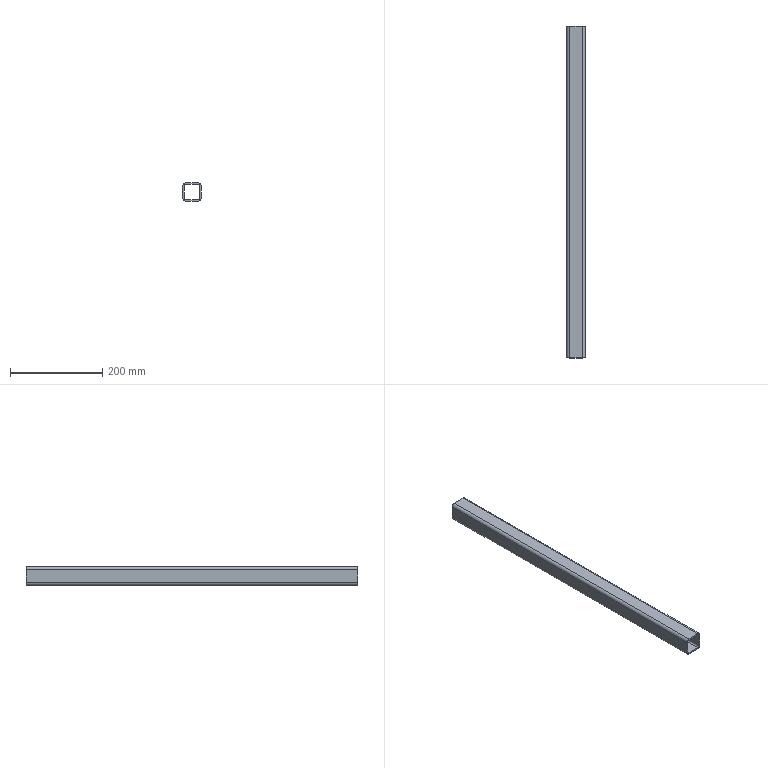Part | SolidWorks | features SavedExtBody 1 | 1 solid | 18 faces | box 40 x 720 x 40 mm | volume 320162 mm3 | plane 10 | cylinder 8 | commonest cylinder face diameters 6.4 x4 12.8 x4
STEP:
#1=CARTESIAN_POINT('',(13.6,400.,-410.));
#2=VERTEX_POINT('',#1);
#3=CARTESIAN_POINT('',(20.,400.,-416.4));
#4=VERTEX_POINT('',#3);
#5=CARTESIAN_POINT('',(13.6,400.,-416.4));
#6=DIRECTION('',(0.,1.,0.));
#7=DIRECTION('',(0.,0.,1.));
#8=AXIS2_PLACEMENT_3D('',#5,#6,#7);
#9=CIRCLE('',#8,6.4);
#10=EDGE_CURVE('',#2,#4,#9,.T.);
#11=ORIENTED_EDGE('',*,*,#10,.F.);
#12=CARTESIAN_POINT('',(13.6,-320.,-410.));
#13=VERTEX_POINT('',#12);
#14=CARTESIAN_POINT('',(13.6,-320.,-410.));
#15=DIRECTION('',(0.,1.,0.));
#16=VECTOR('',#15,1000.);
#17=LINE('',#14,#16);
#18=EDGE_CURVE('',#13,#2,#17,.T.);
#19=ORIENTED_EDGE('',*,*,#18,.F.);
#20=CARTESIAN_POINT('',(20.,-320.,-416.4));
#21=VERTEX_POINT('',#20);
#22=CARTESIAN_POINT('',(13.6,-320.,-416.4));
#23=DIRECTION('',(0.,-1.,0.));
#24=DIRECTION('',(1.,0.,0.));
#25=AXIS2_PLACEMENT_3D('',#22,#23,#24);
#26=CIRCLE('',#25,6.4);
#27=EDGE_CURVE('',#21,#13,#26,.T.);
#28=ORIENTED_EDGE('',*,*,#27,.F.);
#29=CARTESIAN_POINT('',(20.,-320.,-416.4));
#30=DIRECTION('',(0.,1.,0.));
#31=VECTOR('',#30,1000.);
#32=LINE('',#29,#31);
#33=EDGE_CURVE('',#21,#4,#32,.T.);
#34=ORIENTED_EDGE('',*,*,#33,.T.);
#35=EDGE_LOOP('',(#11,#19,#28,#34));
#36=FACE_OUTER_BOUND('',#35,.T.);
#37=CARTESIAN_POINT('',(13.6,-320.,-416.4));
#38=DIRECTION('',(0.,1.,0.));
#39=DIRECTION('',(0.,0.,1.));
#40=AXIS2_PLACEMENT_3D('',#37,#38,#39);
#41=CYLINDRICAL_SURFACE('',#40,6.4);
#42=ADVANCED_FACE('',(#36),#41,.T.);
#43=CARTESIAN_POINT('',(-13.6,400.,-410.));
#44=VERTEX_POINT('',#43);
#45=CARTESIAN_POINT('',(13.6,400.,-410.));
#46=DIRECTION('',(1.,0.,0.));
#47=VECTOR('',#46,1000.);
#48=LINE('',#45,#47);
#49=EDGE_CURVE('',#44,#2,#48,.T.);
#50=ORIENTED_EDGE('',*,*,#49,.F.);
#51=CARTESIAN_POINT('',(-13.6,-320.,-410.));
#52=VERTEX_POINT('',#51);
#53=CARTESIAN_POINT('',(-13.6,-320.,-410.));
#54=DIRECTION('',(0.,1.,0.));
#55=VECTOR('',#54,1000.);
#56=LINE('',#53,#55);
#57=EDGE_CURVE('',#52,#44,#56,.T.);
#58=ORIENTED_EDGE('',*,*,#57,.F.);
#59=CARTESIAN_POINT('',(13.6,-320.,-410.));
#60=DIRECTION('',(-1.,0.,0.));
#61=VECTOR('',#60,1000.);
#62=LINE('',#59,#61);
#63=EDGE_CURVE('',#13,#52,#62,.T.);
#64=ORIENTED_EDGE('',*,*,#63,.F.);
#65=ORIENTED_EDGE('',*,*,#18,.T.);
#66=EDGE_LOOP('',(#50,#58,#64,#65));
#67=FACE_OUTER_BOUND('',#66,.T.);
#68=CARTESIAN_POINT('',(13.6,-320.,-410.));
#69=DIRECTION('',(0.,0.,-1.));
#70=DIRECTION('',(0.,1.,0.));
#71=AXIS2_PLACEMENT_3D('',#68,#69,#70);
#72=PLANE('',#71);
#73=ADVANCED_FACE('',(#67),#72,.F.);
#74=CARTESIAN_POINT('',(-20.,400.,-416.4));
#75=VERTEX_POINT('',#74);
#76=CARTESIAN_POINT('',(-13.6,400.,-416.4));
#77=DIRECTION('',(0.,1.,0.));
#78=DIRECTION('',(0.,0.,1.));
#79=AXIS2_PLACEMENT_3D('',#76,#77,#78);
#80=CIRCLE('',#79,6.4);
#81=EDGE_CURVE('',#75,#44,#80,.T.);
#82=ORIENTED_EDGE('',*,*,#81,.F.);
#83=CARTESIAN_POINT('',(-20.,-320.,-416.4));
#84=VERTEX_POINT('',#83);
#85=CARTESIAN_POINT('',(-20.,-320.,-416.4));
#86=DIRECTION('',(0.,1.,0.));
#87=VECTOR('',#86,1000.);
#88=LINE('',#85,#87);
#89=EDGE_CURVE('',#84,#75,#88,.T.);
#90=ORIENTED_EDGE('',*,*,#89,.F.);
#91=CARTESIAN_POINT('',(-13.6,-320.,-416.4));
#92=DIRECTION('',(0.,-1.,0.));
#93=DIRECTION('',(1.,0.,0.));
#94=AXIS2_PLACEMENT_3D('',#91,#92,#93);
#95=CIRCLE('',#94,6.4);
#96=EDGE_CURVE('',#52,#84,#95,.T.);
#97=ORIENTED_EDGE('',*,*,#96,.F.);
#98=ORIENTED_EDGE('',*,*,#57,.T.);
#99=EDGE_LOOP('',(#82,#90,#97,#98));
#100=FACE_OUTER_BOUND('',#99,.T.);
#101=CARTESIAN_POINT('',(-13.6,-320.,-416.4));
#102=DIRECTION('',(0.,1.,0.));
#103=DIRECTION('',(0.,0.,1.));
#104=AXIS2_PLACEMENT_3D('',#101,#102,#103);
#105=CYLINDRICAL_SURFACE('',#104,6.4);
#106=ADVANCED_FACE('',(#100),#105,.T.);
#107=CARTESIAN_POINT('',(-20.,400.,-443.6));
#108=VERTEX_POINT('',#107);
#109=CARTESIAN_POINT('',(-20.,400.,-443.6));
#110=DIRECTION('',(0.,0.,1.));
#111=VECTOR('',#110,1000.);
#112=LINE('',#109,#111);
#113=EDGE_CURVE('',#108,#75,#112,.T.);
#114=ORIENTED_EDGE('',*,*,#113,.F.);
#115=CARTESIAN_POINT('',(-20.,-320.,-443.6));
#116=VERTEX_POINT('',#115);
#117=CARTESIAN_POINT('',(-20.,-320.,-443.6));
#118=DIRECTION('',(0.,1.,0.));
#119=VECTOR('',#118,1000.);
#120=LINE('',#117,#119);
#121=EDGE_CURVE('',#116,#108,#120,.T.);
#122=ORIENTED_EDGE('',*,*,#121,.F.);
#123=CARTESIAN_POINT('',(-20.,-320.,-443.6));
#124=DIRECTION('',(0.,0.,-1.));
#125=VECTOR('',#124,1000.);
#126=LINE('',#123,#125);
#127=EDGE_CURVE('',#84,#116,#126,.T.);
#128=ORIENTED_EDGE('',*,*,#127,.F.);
#129=ORIENTED_EDGE('',*,*,#89,.T.);
#130=EDGE_LOOP('',(#114,#122,#128,#129));
#131=FACE_OUTER_BOUND('',#130,.T.);
#132=CARTESIAN_POINT('',(-20.,-320.,-443.6));
#133=DIRECTION('',(1.,0.,0.));
#134=DIRECTION('',(0.,0.,-1.));
#135=AXIS2_PLACEMENT_3D('',#132,#133,#134);
#136=PLANE('',#135);
#137=ADVANCED_FACE('',(#131),#136,.F.);
#138=CARTESIAN_POINT('',(-13.6,400.,-450.));
#139=VERTEX_POINT('',#138);
#140=CARTESIAN_POINT('',(-13.6,400.,-443.6));
#141=DIRECTION('',(0.,1.,0.));
#142=DIRECTION('',(0.,0.,1.));
#143=AXIS2_PLACEMENT_3D('',#140,#141,#142);
#144=CIRCLE('',#143,6.4);
#145=EDGE_CURVE('',#139,#108,#144,.T.);
#146=ORIENTED_EDGE('',*,*,#145,.F.);
#147=CARTESIAN_POINT('',(-13.6,-320.,-450.));
#148=VERTEX_POINT('',#147);
#149=CARTESIAN_POINT('',(-13.6,-320.,-450.));
#150=DIRECTION('',(0.,1.,0.));
#151=VECTOR('',#150,1000.);
#152=LINE('',#149,#151);
#153=EDGE_CURVE('',#148,#139,#152,.T.);
#154=ORIENTED_EDGE('',*,*,#153,.F.);
#155=CARTESIAN_POINT('',(-13.6,-320.,-443.6));
#156=DIRECTION('',(0.,-1.,0.));
#157=DIRECTION('',(1.,0.,0.));
#158=AXIS2_PLACEMENT_3D('',#155,#156,#157);
#159=CIRCLE('',#158,6.4);
#160=EDGE_CURVE('',#116,#148,#159,.T.);
#161=ORIENTED_EDGE('',*,*,#160,.F.);
#162=ORIENTED_EDGE('',*,*,#121,.T.);
#163=EDGE_LOOP('',(#146,#154,#161,#162));
#164=FACE_OUTER_BOUND('',#163,.T.);
#165=CARTESIAN_POINT('',(-13.6,-320.,-443.6));
#166=DIRECTION('',(0.,1.,0.));
#167=DIRECTION('',(0.,0.,1.));
#168=AXIS2_PLACEMENT_3D('',#165,#166,#167);
#169=CYLINDRICAL_SURFACE('',#168,6.4);
#170=ADVANCED_FACE('',(#164),#169,.T.);
#171=CARTESIAN_POINT('',(13.6,400.,-450.));
#172=VERTEX_POINT('',#171);
#173=CARTESIAN_POINT('',(0.,400.,-450.));
#174=DIRECTION('',(-1.,0.,0.));
#175=VECTOR('',#174,1000.);
#176=LINE('',#173,#175);
#177=EDGE_CURVE('',#172,#139,#176,.T.);
#178=ORIENTED_EDGE('',*,*,#177,.F.);
#179=CARTESIAN_POINT('',(13.6,-320.,-450.));
#180=VERTEX_POINT('',#179);
#181=CARTESIAN_POINT('',(13.6,-320.,-450.));
#182=DIRECTION('',(0.,1.,0.));
#183=VECTOR('',#182,1000.);
#184=LINE('',#181,#183);
#185=EDGE_CURVE('',#180,#172,#184,.T.);
#186=ORIENTED_EDGE('',*,*,#185,.F.);
#187=CARTESIAN_POINT('',(-13.6,-320.,-450.));
#188=DIRECTION('',(1.,0.,0.));
#189=VECTOR('',#188,1000.);
#190=LINE('',#187,#189);
#191=EDGE_CURVE('',#148,#180,#190,.T.);
#192=ORIENTED_EDGE('',*,*,#191,.F.);
#193=ORIENTED_EDGE('',*,*,#153,.T.);
#194=EDGE_LOOP('',(#178,#186,#192,#193));
#195=FACE_OUTER_BOUND('',#194,.T.);
#196=CARTESIAN_POINT('',(-13.6,-320.,-450.));
#197=DIRECTION('',(0.,0.,1.));
#198=DIRECTION('',(0.,-1.,0.));
#199=AXIS2_PLACEMENT_3D('',#196,#197,#198);
#200=PLANE('',#199);
#201=ADVANCED_FACE('',(#195),#200,.F.);
#202=CARTESIAN_POINT('',(20.,400.,-443.6));
#203=VERTEX_POINT('',#202);
#204=CARTESIAN_POINT('',(13.6,400.,-443.6));
#205=DIRECTION('',(0.,1.,0.));
#206=DIRECTION('',(0.,0.,1.));
#207=AXIS2_PLACEMENT_3D('',#204,#205,#206);
#208=CIRCLE('',#207,6.4);
#209=EDGE_CURVE('',#203,#172,#208,.T.);
#210=ORIENTED_EDGE('',*,*,#209,.F.);
#211=CARTESIAN_POINT('',(20.,-320.,-443.6));
#212=VERTEX_POINT('',#211);
#213=CARTESIAN_POINT('',(20.,-320.,-443.6));
#214=DIRECTION('',(0.,1.,0.));
#215=VECTOR('',#214,1000.);
#216=LINE('',#213,#215);
#217=EDGE_CURVE('',#212,#203,#216,.T.);
#218=ORIENTED_EDGE('',*,*,#217,.F.);
#219=CARTESIAN_POINT('',(13.6,-320.,-443.6));
#220=DIRECTION('',(0.,-1.,0.));
#221=DIRECTION('',(1.,0.,0.));
#222=AXIS2_PLACEMENT_3D('',#219,#220,#221);
#223=CIRCLE('',#222,6.4);
#224=EDGE_CURVE('',#180,#212,#223,.T.);
#225=ORIENTED_EDGE('',*,*,#224,.F.);
#226=ORIENTED_EDGE('',*,*,#185,.T.);
#227=EDGE_LOOP('',(#210,#218,#225,#226));
#228=FACE_OUTER_BOUND('',#227,.T.);
#229=CARTESIAN_POINT('',(13.6,-320.,-443.6));
#230=DIRECTION('',(0.,1.,0.));
#231=DIRECTION('',(0.,0.,1.));
#232=AXIS2_PLACEMENT_3D('',#229,#230,#231);
#233=CYLINDRICAL_SURFACE('',#232,6.4);
#234=ADVANCED_FACE('',(#228),#233,.T.);
#235=CARTESIAN_POINT('',(-16.8,-320.,-416.4));
#236=VERTEX_POINT('',#235);
#237=CARTESIAN_POINT('',(-16.8,400.,-416.4));
#238=VERTEX_POINT('',#237);
#239=CARTESIAN_POINT('',(-16.8,-320.,-416.4));
#240=DIRECTION('',(0.,1.,0.));
#241=VECTOR('',#240,1000.);
#242=LINE('',#239,#241);
#243=EDGE_CURVE('',#236,#238,#242,.T.);
#244=ORIENTED_EDGE('',*,*,#243,.T.);
#245=CARTESIAN_POINT('',(-13.6,400.,-413.2));
#246=VERTEX_POINT('',#245);
#247=CARTESIAN_POINT('',(-13.6,400.,-416.4));
#248=DIRECTION('',(0.,1.,0.));
#249=DIRECTION('',(0.,0.,1.));
#250=AXIS2_PLACEMENT_3D('',#247,#248,#249);
#251=CIRCLE('',#250,3.2);
#252=EDGE_CURVE('',#238,#246,#251,.T.);
#253=ORIENTED_EDGE('',*,*,#252,.T.);
#254=CARTESIAN_POINT('',(-13.6,-320.,-413.2));
#255=VERTEX_POINT('',#254);
#256=CARTESIAN_POINT('',(-13.6,-320.,-413.2));
#257=DIRECTION('',(0.,1.,0.));
#258=VECTOR('',#257,1000.);
#259=LINE('',#256,#258);
#260=EDGE_CURVE('',#255,#246,#259,.T.);
#261=ORIENTED_EDGE('',*,*,#260,.F.);
#262=CARTESIAN_POINT('',(-13.6,-320.,-416.4));
#263=DIRECTION('',(0.,-1.,0.));
#264=DIRECTION('',(1.,0.,0.));
#265=AXIS2_PLACEMENT_3D('',#262,#263,#264);
#266=CIRCLE('',#265,3.2);
#267=EDGE_CURVE('',#255,#236,#266,.T.);
#268=ORIENTED_EDGE('',*,*,#267,.T.);
#269=EDGE_LOOP('',(#244,#253,#261,#268));
#270=FACE_OUTER_BOUND('',#269,.T.);
#271=CARTESIAN_POINT('',(-13.6,-320.,-416.4));
#272=DIRECTION('',(0.,1.,0.));
#273=DIRECTION('',(0.,0.,1.));
#274=AXIS2_PLACEMENT_3D('',#271,#272,#273);
#275=CYLINDRICAL_SURFACE('',#274,3.2);
#276=ADVANCED_FACE('',(#270),#275,.F.);
#277=ORIENTED_EDGE('',*,*,#260,.T.);
#278=CARTESIAN_POINT('',(13.6,400.,-413.2));
#279=VERTEX_POINT('',#278);
#280=CARTESIAN_POINT('',(13.6,400.,-413.2));
#281=DIRECTION('',(1.,0.,0.));
#282=VECTOR('',#281,1000.);
#283=LINE('',#280,#282);
#284=EDGE_CURVE('',#246,#279,#283,.T.);
#285=ORIENTED_EDGE('',*,*,#284,.T.);
#286=CARTESIAN_POINT('',(13.6,-320.,-413.2));
#287=VERTEX_POINT('',#286);
#288=CARTESIAN_POINT('',(13.6,-320.,-413.2));
#289=DIRECTION('',(0.,1.,0.));
#290=VECTOR('',#289,1000.);
#291=LINE('',#288,#290);
#292=EDGE_CURVE('',#287,#279,#291,.T.);
#293=ORIENTED_EDGE('',*,*,#292,.F.);
#294=CARTESIAN_POINT('',(13.6,-320.,-413.2));
#295=DIRECTION('',(-1.,0.,0.));
#296=VECTOR('',#295,1000.);
#297=LINE('',#294,#296);
#298=EDGE_CURVE('',#287,#255,#297,.T.);
#299=ORIENTED_EDGE('',*,*,#298,.T.);
#300=EDGE_LOOP('',(#277,#285,#293,#299));
#301=FACE_OUTER_BOUND('',#300,.T.);
#302=CARTESIAN_POINT('',(13.6,-320.,-413.2));
#303=DIRECTION('',(0.,0.,-1.));
#304=DIRECTION('',(0.,1.,0.));
#305=AXIS2_PLACEMENT_3D('',#302,#303,#304);
#306=PLANE('',#305);
#307=ADVANCED_FACE('',(#301),#306,.T.);
#308=ORIENTED_EDGE('',*,*,#292,.T.);
#309=CARTESIAN_POINT('',(16.8,400.,-416.4));
#310=VERTEX_POINT('',#309);
#311=CARTESIAN_POINT('',(13.6,400.,-416.4));
#312=DIRECTION('',(0.,1.,0.));
#313=DIRECTION('',(0.,0.,1.));
#314=AXIS2_PLACEMENT_3D('',#311,#312,#313);
#315=CIRCLE('',#314,3.2);
#316=EDGE_CURVE('',#279,#310,#315,.T.);
#317=ORIENTED_EDGE('',*,*,#316,.T.);
#318=CARTESIAN_POINT('',(16.8,-320.,-416.4));
#319=VERTEX_POINT('',#318);
#320=CARTESIAN_POINT('',(16.8,-320.,-416.4));
#321=DIRECTION('',(0.,1.,0.));
#322=VECTOR('',#321,1000.);
#323=LINE('',#320,#322);
#324=EDGE_CURVE('',#319,#310,#323,.T.);
#325=ORIENTED_EDGE('',*,*,#324,.F.);
#326=CARTESIAN_POINT('',(13.6,-320.,-416.4));
#327=DIRECTION('',(0.,-1.,0.));
#328=DIRECTION('',(1.,0.,0.));
#329=AXIS2_PLACEMENT_3D('',#326,#327,#328);
#330=CIRCLE('',#329,3.2);
#331=EDGE_CURVE('',#319,#287,#330,.T.);
#332=ORIENTED_EDGE('',*,*,#331,.T.);
#333=EDGE_LOOP('',(#308,#317,#325,#332));
#334=FACE_OUTER_BOUND('',#333,.T.);
#335=CARTESIAN_POINT('',(13.6,-320.,-416.4));
#336=DIRECTION('',(0.,1.,0.));
#337=DIRECTION('',(0.,0.,1.));
#338=AXIS2_PLACEMENT_3D('',#335,#336,#337);
#339=CYLINDRICAL_SURFACE('',#338,3.2);
#340=ADVANCED_FACE('',(#334),#339,.F.);
#341=ORIENTED_EDGE('',*,*,#324,.T.);
#342=CARTESIAN_POINT('',(16.8,400.,-443.6));
#343=VERTEX_POINT('',#342);
#344=CARTESIAN_POINT('',(16.8,400.,-416.4));
#345=DIRECTION('',(0.,0.,-1.));
#346=VECTOR('',#345,1000.);
#347=LINE('',#344,#346);
#348=EDGE_CURVE('',#310,#343,#347,.T.);
#349=ORIENTED_EDGE('',*,*,#348,.T.);
#350=CARTESIAN_POINT('',(16.8,-320.,-443.6));
#351=VERTEX_POINT('',#350);
#352=CARTESIAN_POINT('',(16.8,-320.,-443.6));
#353=DIRECTION('',(0.,1.,0.));
#354=VECTOR('',#353,1000.);
#355=LINE('',#352,#354);
#356=EDGE_CURVE('',#351,#343,#355,.T.);
#357=ORIENTED_EDGE('',*,*,#356,.F.);
#358=CARTESIAN_POINT('',(16.8,-320.,-416.4));
#359=DIRECTION('',(0.,0.,1.));
#360=VECTOR('',#359,1000.);
#361=LINE('',#358,#360);
#362=EDGE_CURVE('',#351,#319,#361,.T.);
#363=ORIENTED_EDGE('',*,*,#362,.T.);
#364=EDGE_LOOP('',(#341,#349,#357,#363));
#365=FACE_OUTER_BOUND('',#364,.T.);
#366=CARTESIAN_POINT('',(16.8,-320.,-416.4));
#367=DIRECTION('',(-1.,0.,0.));
#368=DIRECTION('',(0.,0.,1.));
#369=AXIS2_PLACEMENT_3D('',#366,#367,#368);
#370=PLANE('',#369);
#371=ADVANCED_FACE('',(#365),#370,.T.);
#372=ORIENTED_EDGE('',*,*,#356,.T.);
#373=CARTESIAN_POINT('',(13.6,400.,-446.8));
#374=VERTEX_POINT('',#373);
#375=CARTESIAN_POINT('',(13.6,400.,-443.6));
#376=DIRECTION('',(0.,1.,0.));
#377=DIRECTION('',(0.,0.,1.));
#378=AXIS2_PLACEMENT_3D('',#375,#376,#377);
#379=CIRCLE('',#378,3.2);
#380=EDGE_CURVE('',#343,#374,#379,.T.);
#381=ORIENTED_EDGE('',*,*,#380,.T.);
#382=CARTESIAN_POINT('',(13.6,-320.,-446.8));
#383=VERTEX_POINT('',#382);
#384=CARTESIAN_POINT('',(13.6,-320.,-446.8));
#385=DIRECTION('',(0.,1.,0.));
#386=VECTOR('',#385,1000.);
#387=LINE('',#384,#386);
#388=EDGE_CURVE('',#383,#374,#387,.T.);
#389=ORIENTED_EDGE('',*,*,#388,.F.);
#390=CARTESIAN_POINT('',(13.6,-320.,-443.6));
#391=DIRECTION('',(0.,-1.,0.));
#392=DIRECTION('',(1.,0.,0.));
#393=AXIS2_PLACEMENT_3D('',#390,#391,#392);
#394=CIRCLE('',#393,3.2);
#395=EDGE_CURVE('',#383,#351,#394,.T.);
#396=ORIENTED_EDGE('',*,*,#395,.T.);
#397=EDGE_LOOP('',(#372,#381,#389,#396));
#398=FACE_OUTER_BOUND('',#397,.T.);
#399=CARTESIAN_POINT('',(13.6,-320.,-443.6));
#400=DIRECTION('',(0.,1.,0.));
#401=DIRECTION('',(0.,0.,1.));
#402=AXIS2_PLACEMENT_3D('',#399,#400,#401);
#403=CYLINDRICAL_SURFACE('',#402,3.2);
#404=ADVANCED_FACE('',(#398),#403,.F.);
#405=ORIENTED_EDGE('',*,*,#388,.T.);
#406=CARTESIAN_POINT('',(-13.6,400.,-446.8));
#407=VERTEX_POINT('',#406);
#408=CARTESIAN_POINT('',(-13.6,400.,-446.8));
#409=DIRECTION('',(-1.,0.,0.));
#410=VECTOR('',#409,1000.);
#411=LINE('',#408,#410);
#412=EDGE_CURVE('',#374,#407,#411,.T.);
#413=ORIENTED_EDGE('',*,*,#412,.T.);
#414=CARTESIAN_POINT('',(-13.6,-320.,-446.8));
#415=VERTEX_POINT('',#414);
#416=CARTESIAN_POINT('',(-13.6,-320.,-446.8));
#417=DIRECTION('',(0.,1.,0.));
#418=VECTOR('',#417,1000.);
#419=LINE('',#416,#418);
#420=EDGE_CURVE('',#415,#407,#419,.T.);
#421=ORIENTED_EDGE('',*,*,#420,.F.);
#422=CARTESIAN_POINT('',(-13.6,-320.,-446.8));
#423=DIRECTION('',(1.,0.,0.));
#424=VECTOR('',#423,1000.);
#425=LINE('',#422,#424);
#426=EDGE_CURVE('',#415,#383,#425,.T.);
#427=ORIENTED_EDGE('',*,*,#426,.T.);
#428=EDGE_LOOP('',(#405,#413,#421,#427));
#429=FACE_OUTER_BOUND('',#428,.T.);
#430=CARTESIAN_POINT('',(-13.6,-320.,-446.8));
#431=DIRECTION('',(0.,0.,1.));
#432=DIRECTION('',(0.,-1.,0.));
#433=AXIS2_PLACEMENT_3D('',#430,#431,#432);
#434=PLANE('',#433);
#435=ADVANCED_FACE('',(#429),#434,.T.);
#436=ORIENTED_EDGE('',*,*,#420,.T.);
#437=CARTESIAN_POINT('',(-16.8,400.,-443.6));
#438=VERTEX_POINT('',#437);
#439=CARTESIAN_POINT('',(-13.6,400.,-443.6));
#440=DIRECTION('',(0.,1.,0.));
#441=DIRECTION('',(0.,0.,1.));
#442=AXIS2_PLACEMENT_3D('',#439,#440,#441);
#443=CIRCLE('',#442,3.2);
#444=EDGE_CURVE('',#407,#438,#443,.T.);
#445=ORIENTED_EDGE('',*,*,#444,.T.);
#446=CARTESIAN_POINT('',(-16.8,-320.,-443.6));
#447=VERTEX_POINT('',#446);
#448=CARTESIAN_POINT('',(-16.8,-320.,-443.6));
#449=DIRECTION('',(0.,1.,0.));
#450=VECTOR('',#449,1000.);
#451=LINE('',#448,#450);
#452=EDGE_CURVE('',#447,#438,#451,.T.);
#453=ORIENTED_EDGE('',*,*,#452,.F.);
#454=CARTESIAN_POINT('',(-13.6,-320.,-443.6));
#455=DIRECTION('',(0.,-1.,0.));
#456=DIRECTION('',(1.,0.,0.));
#457=AXIS2_PLACEMENT_3D('',#454,#455,#456);
#458=CIRCLE('',#457,3.2);
#459=EDGE_CURVE('',#447,#415,#458,.T.);
#460=ORIENTED_EDGE('',*,*,#459,.T.);
#461=EDGE_LOOP('',(#436,#445,#453,#460));
#462=FACE_OUTER_BOUND('',#461,.T.);
#463=CARTESIAN_POINT('',(-13.6,-320.,-443.6));
#464=DIRECTION('',(0.,1.,0.));
#465=DIRECTION('',(0.,0.,1.));
#466=AXIS2_PLACEMENT_3D('',#463,#464,#465);
#467=CYLINDRICAL_SURFACE('',#466,3.2);
#468=ADVANCED_FACE('',(#462),#467,.F.);
#469=ORIENTED_EDGE('',*,*,#452,.T.);
#470=CARTESIAN_POINT('',(-16.8,400.,-443.6));
#471=DIRECTION('',(0.,0.,1.));
#472=VECTOR('',#471,1000.);
#473=LINE('',#470,#472);
#474=EDGE_CURVE('',#438,#238,#473,.T.);
#475=ORIENTED_EDGE('',*,*,#474,.T.);
#476=ORIENTED_EDGE('',*,*,#243,.F.);
#477=CARTESIAN_POINT('',(-16.8,-320.,-443.6));
#478=DIRECTION('',(0.,0.,-1.));
#479=VECTOR('',#478,1000.);
#480=LINE('',#477,#479);
#481=EDGE_CURVE('',#236,#447,#480,.T.);
#482=ORIENTED_EDGE('',*,*,#481,.T.);
#483=EDGE_LOOP('',(#469,#475,#476,#482));
#484=FACE_OUTER_BOUND('',#483,.T.);
#485=CARTESIAN_POINT('',(-16.8,-320.,-443.6));
#486=DIRECTION('',(1.,0.,0.));
#487=DIRECTION('',(0.,0.,-1.));
#488=AXIS2_PLACEMENT_3D('',#485,#486,#487);
#489=PLANE('',#488);
#490=ADVANCED_FACE('',(#484),#489,.T.);
#491=CARTESIAN_POINT('',(20.,400.,-416.4));
#492=DIRECTION('',(0.,0.,-1.));
#493=VECTOR('',#492,1000.);
#494=LINE('',#491,#493);
#495=EDGE_CURVE('',#4,#203,#494,.T.);
#496=ORIENTED_EDGE('',*,*,#495,.F.);
#497=ORIENTED_EDGE('',*,*,#33,.F.);
#498=CARTESIAN_POINT('',(20.,-320.,-416.4));
#499=DIRECTION('',(0.,0.,1.));
#500=VECTOR('',#499,1000.);
#501=LINE('',#498,#500);
#502=EDGE_CURVE('',#212,#21,#501,.T.);
#503=ORIENTED_EDGE('',*,*,#502,.F.);
#504=ORIENTED_EDGE('',*,*,#217,.T.);
#505=EDGE_LOOP('',(#496,#497,#503,#504));
#506=FACE_OUTER_BOUND('',#505,.T.);
#507=CARTESIAN_POINT('',(20.,-320.,-416.4));
#508=DIRECTION('',(-1.,0.,0.));
#509=DIRECTION('',(0.,0.,1.));
#510=AXIS2_PLACEMENT_3D('',#507,#508,#509);
#511=PLANE('',#510);
#512=ADVANCED_FACE('',(#506),#511,.F.);
#513=ORIENTED_EDGE('',*,*,#267,.F.);
#514=ORIENTED_EDGE('',*,*,#298,.F.);
#515=ORIENTED_EDGE('',*,*,#331,.F.);
#516=ORIENTED_EDGE('',*,*,#362,.F.);
#517=ORIENTED_EDGE('',*,*,#395,.F.);
#518=ORIENTED_EDGE('',*,*,#426,.F.);
#519=ORIENTED_EDGE('',*,*,#459,.F.);
#520=ORIENTED_EDGE('',*,*,#481,.F.);
#521=EDGE_LOOP('',(#513,#514,#515,#516,#517,#518,#519,#520));
#522=FACE_BOUND('',#521,.T.);
#523=ORIENTED_EDGE('',*,*,#27,.T.);
#524=ORIENTED_EDGE('',*,*,#63,.T.);
#525=ORIENTED_EDGE('',*,*,#96,.T.);
#526=ORIENTED_EDGE('',*,*,#127,.T.);
#527=ORIENTED_EDGE('',*,*,#160,.T.);
#528=ORIENTED_EDGE('',*,*,#191,.T.);
#529=ORIENTED_EDGE('',*,*,#224,.T.);
#530=ORIENTED_EDGE('',*,*,#502,.T.);
#531=EDGE_LOOP('',(#523,#524,#525,#526,#527,#528,#529,#530));
#532=FACE_OUTER_BOUND('',#531,.T.);
#533=CARTESIAN_POINT('',(13.6,-320.,-416.4));
#534=DIRECTION('',(0.,-1.,0.));
#535=DIRECTION('',(1.,0.,0.));
#536=AXIS2_PLACEMENT_3D('',#533,#534,#535);
#537=PLANE('',#536);
#538=ADVANCED_FACE('',(#522,#532),#537,.T.);
#539=ORIENTED_EDGE('',*,*,#474,.F.);
#540=ORIENTED_EDGE('',*,*,#444,.F.);
#541=ORIENTED_EDGE('',*,*,#412,.F.);
#542=ORIENTED_EDGE('',*,*,#380,.F.);
#543=ORIENTED_EDGE('',*,*,#348,.F.);
#544=ORIENTED_EDGE('',*,*,#316,.F.);
#545=ORIENTED_EDGE('',*,*,#284,.F.);
#546=ORIENTED_EDGE('',*,*,#252,.F.);
#547=EDGE_LOOP('',(#539,#540,#541,#542,#543,#544,#545,#546));
#548=FACE_BOUND('',#547,.T.);
#549=ORIENTED_EDGE('',*,*,#10,.T.);
#550=ORIENTED_EDGE('',*,*,#495,.T.);
#551=ORIENTED_EDGE('',*,*,#209,.T.);
#552=ORIENTED_EDGE('',*,*,#177,.T.);
#553=ORIENTED_EDGE('',*,*,#145,.T.);
#554=ORIENTED_EDGE('',*,*,#113,.T.);
#555=ORIENTED_EDGE('',*,*,#81,.T.);
#556=ORIENTED_EDGE('',*,*,#49,.T.);
#557=EDGE_LOOP('',(#549,#550,#551,#552,#553,#554,#555,#556));
#558=FACE_OUTER_BOUND('',#557,.T.);
#559=CARTESIAN_POINT('',(0.,400.,-416.4));
#560=DIRECTION('',(0.,1.,0.));
#561=DIRECTION('',(0.,0.,1.));
#562=AXIS2_PLACEMENT_3D('',#559,#560,#561);
#563=PLANE('',#562);
#564=ADVANCED_FACE('',(#548,#558),#563,.T.);
#565=CLOSED_SHELL('',(#42,#73,#106,#137,#170,#201,#234,#276,#307,#340,#371,#404,#435,#468,#490,#512,#538,#564));
#566=MANIFOLD_SOLID_BREP('',#565);
#567=CARTESIAN_POINT('',(0.,0.,0.));
#568=DIRECTION('',(0.,0.,1.));
#569=DIRECTION('',(1.,0.,0.));
#570=AXIS2_PLACEMENT_3D('',#567,#568,#569);
#571=(LENGTH_UNIT()NAMED_UNIT(*)SI_UNIT(.MILLI.,.METRE.));
#572=UNCERTAINTY_MEASURE_WITH_UNIT(LENGTH_MEASURE(0.00001),#571,'','');
#573=(NAMED_UNIT(*)PLANE_ANGLE_UNIT()SI_UNIT($,.RADIAN.));
#574=(NAMED_UNIT(*)SI_UNIT($,.STERADIAN.)SOLID_ANGLE_UNIT());
#575=(GEOMETRIC_REPRESENTATION_CONTEXT(3)GLOBAL_UNCERTAINTY_ASSIGNED_CONTEXT((#572))GLOBAL_UNIT_ASSIGNED_CONTEXT((#571,#573,#574))REPRESENTATION_CONTEXT('',''));
#576=ADVANCED_BREP_SHAPE_REPRESENTATION('',(#566,#570),#575);